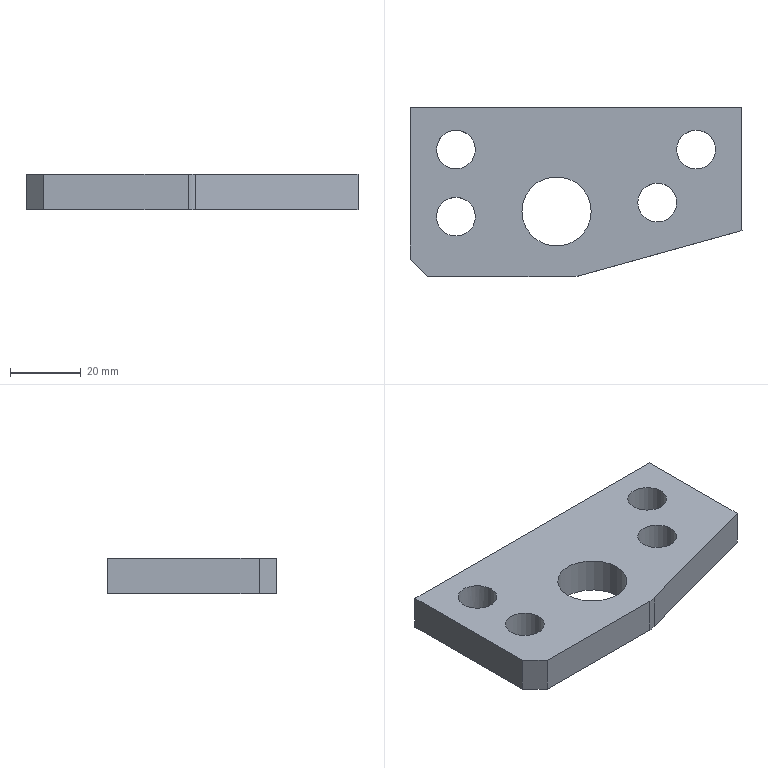Part | STEP file | lll_id4514_x_t | 1 solid | 14 faces | box 94 x 48 x 10 mm | volume 35108 mm3 | plane 8 | cylinder 6 | commonest cylinder face diameters 11 x4 16 x1 19.6 x1
STEP:
#1=CARTESIAN_POINT('',(3558.734,-207.45,-35.));
#2=VERTEX_POINT('',#1);
#3=CARTESIAN_POINT('',(3558.734,-212.95,-35.));
#4=DIRECTION('',(0.,0.,1.));
#5=DIRECTION('',(0.,1.,0.));
#6=AXIS2_PLACEMENT_3D('',#3,#4,#5);
#7=CIRCLE('',#6,5.5);
#8=EDGE_CURVE('',#2,#2,#7,.T.);
#9=ORIENTED_EDGE('',*,*,#8,.F.);
#10=EDGE_LOOP('',(#9));
#11=FACE_BOUND('',#10,.T.);
#12=CARTESIAN_POINT('',(3545.734,-200.95,-35.));
#13=VERTEX_POINT('',#12);
#14=CARTESIAN_POINT('',(3545.734,-243.95,-35.));
#15=VERTEX_POINT('',#14);
#16=CARTESIAN_POINT('',(3545.734,-198.7,-35.));
#17=DIRECTION('',(0.,-1.,0.));
#18=VECTOR('',#17,1.);
#19=LINE('',#16,#18);
#20=EDGE_CURVE('',#13,#15,#19,.T.);
#21=ORIENTED_EDGE('',*,*,#20,.T.);
#22=CARTESIAN_POINT('',(3550.734,-248.95,-35.));
#23=VERTEX_POINT('',#22);
#24=CARTESIAN_POINT('',(3540.359,-238.575,-35.));
#25=DIRECTION('',(0.7071,-0.7071,0.));
#26=VECTOR('',#25,1.);
#27=LINE('',#24,#26);
#28=EDGE_CURVE('',#15,#23,#27,.T.);
#29=ORIENTED_EDGE('',*,*,#28,.T.);
#30=CARTESIAN_POINT('',(3591.644,-248.95,-35.));
#31=VERTEX_POINT('',#30);
#32=CARTESIAN_POINT('',(3580.234,-248.95,-35.));
#33=DIRECTION('',(1.,0.,0.));
#34=VECTOR('',#33,1.);
#35=LINE('',#32,#34);
#36=EDGE_CURVE('',#23,#31,#35,.T.);
#37=ORIENTED_EDGE('',*,*,#36,.T.);
#38=CARTESIAN_POINT('',(3593.785,-248.658,-35.));
#39=VERTEX_POINT('',#38);
#40=CARTESIAN_POINT('',(3591.644,-240.95,-35.));
#41=DIRECTION('',(0.,0.,1.));
#42=DIRECTION('',(1.,0.,0.));
#43=AXIS2_PLACEMENT_3D('',#40,#41,#42);
#44=CIRCLE('',#43,8.);
#45=EDGE_CURVE('',#31,#39,#44,.T.);
#46=ORIENTED_EDGE('',*,*,#45,.T.);
#47=CARTESIAN_POINT('',(3639.734,-235.894,-35.));
#48=VERTEX_POINT('',#47);
#49=CARTESIAN_POINT('',(3594.088,-248.574,-35.));
#50=DIRECTION('',(0.9635,0.2676,0.));
#51=VECTOR('',#50,1.);
#52=LINE('',#49,#51);
#53=EDGE_CURVE('',#39,#48,#52,.T.);
#54=ORIENTED_EDGE('',*,*,#53,.T.);
#55=CARTESIAN_POINT('',(3639.734,-200.95,-35.));
#56=VERTEX_POINT('',#55);
#57=CARTESIAN_POINT('',(3639.734,-198.7,-35.));
#58=DIRECTION('',(0.,1.,0.));
#59=VECTOR('',#58,1.);
#60=LINE('',#57,#59);
#61=EDGE_CURVE('',#48,#56,#60,.T.);
#62=ORIENTED_EDGE('',*,*,#61,.T.);
#63=CARTESIAN_POINT('',(3580.234,-200.95,-35.));
#64=DIRECTION('',(-1.,0.,0.));
#65=VECTOR('',#64,1.);
#66=LINE('',#63,#65);
#67=EDGE_CURVE('',#56,#13,#66,.T.);
#68=ORIENTED_EDGE('',*,*,#67,.T.);
#69=EDGE_LOOP('',(#21,#29,#37,#46,#54,#62,#68));
#70=FACE_BOUND('',#69,.T.);
#71=CARTESIAN_POINT('',(3553.234,-231.95,-35.));
#72=VERTEX_POINT('',#71);
#73=CARTESIAN_POINT('',(3558.734,-231.95,-35.));
#74=DIRECTION('',(0.,0.,1.));
#75=DIRECTION('',(-1.,0.,0.));
#76=AXIS2_PLACEMENT_3D('',#73,#74,#75);
#77=CIRCLE('',#76,5.5);
#78=EDGE_CURVE('',#72,#72,#77,.T.);
#79=ORIENTED_EDGE('',*,*,#78,.F.);
#80=EDGE_LOOP('',(#79));
#81=FACE_BOUND('',#80,.T.);
#82=CARTESIAN_POINT('',(3610.234,-227.95,-35.));
#83=VERTEX_POINT('',#82);
#84=CARTESIAN_POINT('',(3615.734,-227.95,-35.));
#85=DIRECTION('',(0.,0.,1.));
#86=DIRECTION('',(-1.,0.,0.));
#87=AXIS2_PLACEMENT_3D('',#84,#85,#86);
#88=CIRCLE('',#87,5.5);
#89=EDGE_CURVE('',#83,#83,#88,.T.);
#90=ORIENTED_EDGE('',*,*,#89,.F.);
#91=EDGE_LOOP('',(#90));
#92=FACE_BOUND('',#91,.T.);
#93=CARTESIAN_POINT('',(3632.234,-212.95,-35.));
#94=VERTEX_POINT('',#93);
#95=CARTESIAN_POINT('',(3626.734,-212.95,-35.));
#96=DIRECTION('',(0.,0.,1.));
#97=DIRECTION('',(1.,0.,0.));
#98=AXIS2_PLACEMENT_3D('',#95,#96,#97);
#99=CIRCLE('',#98,5.5);
#100=EDGE_CURVE('',#94,#94,#99,.T.);
#101=ORIENTED_EDGE('',*,*,#100,.F.);
#102=EDGE_LOOP('',(#101));
#103=FACE_BOUND('',#102,.T.);
#104=CARTESIAN_POINT('',(3597.034,-230.45,-35.));
#105=VERTEX_POINT('',#104);
#106=CARTESIAN_POINT('',(3587.234,-230.45,-35.));
#107=DIRECTION('',(0.,0.,-1.));
#108=DIRECTION('',(1.,0.,0.));
#109=AXIS2_PLACEMENT_3D('',#106,#107,#108);
#110=CIRCLE('',#109,9.8);
#111=EDGE_CURVE('',#105,#105,#110,.T.);
#112=ORIENTED_EDGE('',*,*,#111,.T.);
#113=EDGE_LOOP('',(#112));
#114=FACE_BOUND('',#113,.T.);
#115=CARTESIAN_POINT('',(3580.234,-198.7,-35.));
#116=DIRECTION('',(0.,0.,-1.));
#117=DIRECTION('',(0.,-1.,0.));
#118=AXIS2_PLACEMENT_3D('',#115,#116,#117);
#119=PLANE('',#118);
#120=ADVANCED_FACE('',(#11,#70,#81,#92,#103,#114),#119,.F.);
#121=CARTESIAN_POINT('',(3564.234,-212.95,-45.));
#122=VERTEX_POINT('',#121);
#123=CARTESIAN_POINT('',(3558.734,-212.95,-45.));
#124=DIRECTION('',(0.,0.,1.));
#125=DIRECTION('',(1.,0.,0.));
#126=AXIS2_PLACEMENT_3D('',#123,#124,#125);
#127=CIRCLE('',#126,5.5);
#128=EDGE_CURVE('',#122,#122,#127,.T.);
#129=ORIENTED_EDGE('',*,*,#128,.T.);
#130=EDGE_LOOP('',(#129));
#131=FACE_BOUND('',#130,.T.);
#132=CARTESIAN_POINT('',(3545.734,-200.95,-45.));
#133=VERTEX_POINT('',#132);
#134=CARTESIAN_POINT('',(3545.734,-243.95,-45.));
#135=VERTEX_POINT('',#134);
#136=CARTESIAN_POINT('',(3545.734,-198.7,-45.));
#137=DIRECTION('',(0.,-1.,0.));
#138=VECTOR('',#137,1.);
#139=LINE('',#136,#138);
#140=EDGE_CURVE('',#133,#135,#139,.T.);
#141=ORIENTED_EDGE('',*,*,#140,.F.);
#142=CARTESIAN_POINT('',(3639.734,-200.95,-45.));
#143=VERTEX_POINT('',#142);
#144=CARTESIAN_POINT('',(3580.234,-200.95,-45.));
#145=DIRECTION('',(-1.,0.,0.));
#146=VECTOR('',#145,1.);
#147=LINE('',#144,#146);
#148=EDGE_CURVE('',#143,#133,#147,.T.);
#149=ORIENTED_EDGE('',*,*,#148,.F.);
#150=CARTESIAN_POINT('',(3639.734,-235.894,-45.));
#151=VERTEX_POINT('',#150);
#152=CARTESIAN_POINT('',(3639.734,-198.7,-45.));
#153=DIRECTION('',(0.,1.,0.));
#154=VECTOR('',#153,1.);
#155=LINE('',#152,#154);
#156=EDGE_CURVE('',#151,#143,#155,.T.);
#157=ORIENTED_EDGE('',*,*,#156,.F.);
#158=CARTESIAN_POINT('',(3593.785,-248.658,-45.));
#159=VERTEX_POINT('',#158);
#160=CARTESIAN_POINT('',(3594.088,-248.574,-45.));
#161=DIRECTION('',(0.9635,0.2676,0.));
#162=VECTOR('',#161,1.);
#163=LINE('',#160,#162);
#164=EDGE_CURVE('',#159,#151,#163,.T.);
#165=ORIENTED_EDGE('',*,*,#164,.F.);
#166=CARTESIAN_POINT('',(3591.644,-248.95,-45.));
#167=VERTEX_POINT('',#166);
#168=CARTESIAN_POINT('',(3591.644,-240.95,-45.));
#169=DIRECTION('',(0.,0.,1.));
#170=DIRECTION('',(1.,0.,0.));
#171=AXIS2_PLACEMENT_3D('',#168,#169,#170);
#172=CIRCLE('',#171,8.);
#173=EDGE_CURVE('',#167,#159,#172,.T.);
#174=ORIENTED_EDGE('',*,*,#173,.F.);
#175=CARTESIAN_POINT('',(3550.734,-248.95,-45.));
#176=VERTEX_POINT('',#175);
#177=CARTESIAN_POINT('',(3580.234,-248.95,-45.));
#178=DIRECTION('',(1.,0.,0.));
#179=VECTOR('',#178,1.);
#180=LINE('',#177,#179);
#181=EDGE_CURVE('',#176,#167,#180,.T.);
#182=ORIENTED_EDGE('',*,*,#181,.F.);
#183=CARTESIAN_POINT('',(3540.359,-238.575,-45.));
#184=DIRECTION('',(0.7071,-0.7071,0.));
#185=VECTOR('',#184,1.);
#186=LINE('',#183,#185);
#187=EDGE_CURVE('',#135,#176,#186,.T.);
#188=ORIENTED_EDGE('',*,*,#187,.F.);
#189=EDGE_LOOP('',(#141,#149,#157,#165,#174,#182,#188));
#190=FACE_BOUND('',#189,.T.);
#191=CARTESIAN_POINT('',(3553.234,-231.95,-45.));
#192=VERTEX_POINT('',#191);
#193=CARTESIAN_POINT('',(3558.734,-231.95,-45.));
#194=DIRECTION('',(0.,0.,1.));
#195=DIRECTION('',(-1.,0.,0.));
#196=AXIS2_PLACEMENT_3D('',#193,#194,#195);
#197=CIRCLE('',#196,5.5);
#198=EDGE_CURVE('',#192,#192,#197,.T.);
#199=ORIENTED_EDGE('',*,*,#198,.T.);
#200=EDGE_LOOP('',(#199));
#201=FACE_BOUND('',#200,.T.);
#202=CARTESIAN_POINT('',(3610.234,-227.95,-45.));
#203=VERTEX_POINT('',#202);
#204=CARTESIAN_POINT('',(3615.734,-227.95,-45.));
#205=DIRECTION('',(0.,0.,1.));
#206=DIRECTION('',(-1.,0.,0.));
#207=AXIS2_PLACEMENT_3D('',#204,#205,#206);
#208=CIRCLE('',#207,5.5);
#209=EDGE_CURVE('',#203,#203,#208,.T.);
#210=ORIENTED_EDGE('',*,*,#209,.T.);
#211=EDGE_LOOP('',(#210));
#212=FACE_BOUND('',#211,.T.);
#213=CARTESIAN_POINT('',(3632.234,-212.95,-45.));
#214=VERTEX_POINT('',#213);
#215=CARTESIAN_POINT('',(3626.734,-212.95,-45.));
#216=DIRECTION('',(0.,0.,1.));
#217=DIRECTION('',(1.,0.,0.));
#218=AXIS2_PLACEMENT_3D('',#215,#216,#217);
#219=CIRCLE('',#218,5.5);
#220=EDGE_CURVE('',#214,#214,#219,.T.);
#221=ORIENTED_EDGE('',*,*,#220,.T.);
#222=EDGE_LOOP('',(#221));
#223=FACE_BOUND('',#222,.T.);
#224=CARTESIAN_POINT('',(3597.034,-230.45,-45.));
#225=VERTEX_POINT('',#224);
#226=CARTESIAN_POINT('',(3587.234,-230.45,-45.));
#227=DIRECTION('',(0.,0.,-1.));
#228=DIRECTION('',(1.,0.,0.));
#229=AXIS2_PLACEMENT_3D('',#226,#227,#228);
#230=CIRCLE('',#229,9.8);
#231=EDGE_CURVE('',#225,#225,#230,.T.);
#232=ORIENTED_EDGE('',*,*,#231,.F.);
#233=EDGE_LOOP('',(#232));
#234=FACE_BOUND('',#233,.T.);
#235=CARTESIAN_POINT('',(3580.234,-198.7,-45.));
#236=DIRECTION('',(0.,0.,-1.));
#237=DIRECTION('',(0.,-1.,0.));
#238=AXIS2_PLACEMENT_3D('',#235,#236,#237);
#239=PLANE('',#238);
#240=ADVANCED_FACE('',(#131,#190,#201,#212,#223,#234),#239,.T.);
#241=CARTESIAN_POINT('',(3550.734,-248.95,-35.));
#242=DIRECTION('',(0.,0.,1.));
#243=VECTOR('',#242,1.);
#244=LINE('',#241,#243);
#245=EDGE_CURVE('',#176,#23,#244,.T.);
#246=ORIENTED_EDGE('',*,*,#245,.F.);
#247=ORIENTED_EDGE('',*,*,#181,.T.);
#248=CARTESIAN_POINT('',(3591.644,-248.95,-35.));
#249=DIRECTION('',(0.,0.,1.));
#250=VECTOR('',#249,1.);
#251=LINE('',#248,#250);
#252=EDGE_CURVE('',#167,#31,#251,.T.);
#253=ORIENTED_EDGE('',*,*,#252,.T.);
#254=ORIENTED_EDGE('',*,*,#36,.F.);
#255=EDGE_LOOP('',(#246,#247,#253,#254));
#256=FACE_OUTER_BOUND('',#255,.T.);
#257=CARTESIAN_POINT('',(3580.234,-248.95,-35.));
#258=DIRECTION('',(0.,-1.,0.));
#259=DIRECTION('',(1.,0.,0.));
#260=AXIS2_PLACEMENT_3D('',#257,#258,#259);
#261=PLANE('',#260);
#262=ADVANCED_FACE('',(#256),#261,.T.);
#263=ORIENTED_EDGE('',*,*,#252,.F.);
#264=ORIENTED_EDGE('',*,*,#173,.T.);
#265=CARTESIAN_POINT('',(3593.785,-248.658,-35.));
#266=DIRECTION('',(0.,0.,1.));
#267=VECTOR('',#266,1.);
#268=LINE('',#265,#267);
#269=EDGE_CURVE('',#159,#39,#268,.T.);
#270=ORIENTED_EDGE('',*,*,#269,.T.);
#271=ORIENTED_EDGE('',*,*,#45,.F.);
#272=EDGE_LOOP('',(#263,#264,#270,#271));
#273=FACE_OUTER_BOUND('',#272,.T.);
#274=CARTESIAN_POINT('',(3591.644,-240.95,-35.));
#275=DIRECTION('',(0.,0.,-1.));
#276=DIRECTION('',(1.,0.,0.));
#277=AXIS2_PLACEMENT_3D('',#274,#275,#276);
#278=CYLINDRICAL_SURFACE('',#277,8.);
#279=ADVANCED_FACE('',(#273),#278,.T.);
#280=ORIENTED_EDGE('',*,*,#269,.F.);
#281=ORIENTED_EDGE('',*,*,#164,.T.);
#282=CARTESIAN_POINT('',(3639.734,-235.894,-35.));
#283=DIRECTION('',(0.,0.,1.));
#284=VECTOR('',#283,1.);
#285=LINE('',#282,#284);
#286=EDGE_CURVE('',#151,#48,#285,.T.);
#287=ORIENTED_EDGE('',*,*,#286,.T.);
#288=ORIENTED_EDGE('',*,*,#53,.F.);
#289=EDGE_LOOP('',(#280,#281,#287,#288));
#290=FACE_OUTER_BOUND('',#289,.T.);
#291=CARTESIAN_POINT('',(3594.088,-248.574,-35.));
#292=DIRECTION('',(-0.2676,0.9635,0.));
#293=DIRECTION('',(-0.9635,-0.2676,0.));
#294=AXIS2_PLACEMENT_3D('',#291,#292,#293);
#295=PLANE('',#294);
#296=ADVANCED_FACE('',(#290),#295,.F.);
#297=ORIENTED_EDGE('',*,*,#286,.F.);
#298=ORIENTED_EDGE('',*,*,#156,.T.);
#299=CARTESIAN_POINT('',(3639.734,-200.95,-35.));
#300=DIRECTION('',(0.,0.,1.));
#301=VECTOR('',#300,1.);
#302=LINE('',#299,#301);
#303=EDGE_CURVE('',#143,#56,#302,.T.);
#304=ORIENTED_EDGE('',*,*,#303,.T.);
#305=ORIENTED_EDGE('',*,*,#61,.F.);
#306=EDGE_LOOP('',(#297,#298,#304,#305));
#307=FACE_OUTER_BOUND('',#306,.T.);
#308=CARTESIAN_POINT('',(3639.734,-198.7,-35.));
#309=DIRECTION('',(1.,0.,0.));
#310=DIRECTION('',(0.,1.,0.));
#311=AXIS2_PLACEMENT_3D('',#308,#309,#310);
#312=PLANE('',#311);
#313=ADVANCED_FACE('',(#307),#312,.T.);
#314=ORIENTED_EDGE('',*,*,#303,.F.);
#315=ORIENTED_EDGE('',*,*,#148,.T.);
#316=CARTESIAN_POINT('',(3545.734,-200.95,-35.));
#317=DIRECTION('',(0.,0.,1.));
#318=VECTOR('',#317,1.);
#319=LINE('',#316,#318);
#320=EDGE_CURVE('',#133,#13,#319,.T.);
#321=ORIENTED_EDGE('',*,*,#320,.T.);
#322=ORIENTED_EDGE('',*,*,#67,.F.);
#323=EDGE_LOOP('',(#314,#315,#321,#322));
#324=FACE_OUTER_BOUND('',#323,.T.);
#325=CARTESIAN_POINT('',(3580.234,-200.95,-35.));
#326=DIRECTION('',(0.,1.,0.));
#327=DIRECTION('',(-1.,0.,0.));
#328=AXIS2_PLACEMENT_3D('',#325,#326,#327);
#329=PLANE('',#328);
#330=ADVANCED_FACE('',(#324),#329,.T.);
#331=ORIENTED_EDGE('',*,*,#320,.F.);
#332=ORIENTED_EDGE('',*,*,#140,.T.);
#333=CARTESIAN_POINT('',(3545.734,-243.95,-35.));
#334=DIRECTION('',(0.,0.,1.));
#335=VECTOR('',#334,1.);
#336=LINE('',#333,#335);
#337=EDGE_CURVE('',#135,#15,#336,.T.);
#338=ORIENTED_EDGE('',*,*,#337,.T.);
#339=ORIENTED_EDGE('',*,*,#20,.F.);
#340=EDGE_LOOP('',(#331,#332,#338,#339));
#341=FACE_OUTER_BOUND('',#340,.T.);
#342=CARTESIAN_POINT('',(3545.734,-198.7,-35.));
#343=DIRECTION('',(-1.,0.,0.));
#344=DIRECTION('',(0.,-1.,0.));
#345=AXIS2_PLACEMENT_3D('',#342,#343,#344);
#346=PLANE('',#345);
#347=ADVANCED_FACE('',(#341),#346,.T.);
#348=ORIENTED_EDGE('',*,*,#100,.T.);
#349=EDGE_LOOP('',(#348));
#350=FACE_BOUND('',#349,.T.);
#351=ORIENTED_EDGE('',*,*,#220,.F.);
#352=EDGE_LOOP('',(#351));
#353=FACE_BOUND('',#352,.T.);
#354=CARTESIAN_POINT('',(3626.734,-212.95,-35.));
#355=DIRECTION('',(0.,0.,-1.));
#356=DIRECTION('',(1.,0.,0.));
#357=AXIS2_PLACEMENT_3D('',#354,#355,#356);
#358=CYLINDRICAL_SURFACE('',#357,5.5);
#359=ADVANCED_FACE('',(#350,#353),#358,.F.);
#360=ORIENTED_EDGE('',*,*,#89,.T.);
#361=EDGE_LOOP('',(#360));
#362=FACE_BOUND('',#361,.T.);
#363=ORIENTED_EDGE('',*,*,#209,.F.);
#364=EDGE_LOOP('',(#363));
#365=FACE_BOUND('',#364,.T.);
#366=CARTESIAN_POINT('',(3615.734,-227.95,-35.));
#367=DIRECTION('',(0.,0.,-1.));
#368=DIRECTION('',(1.,0.,0.));
#369=AXIS2_PLACEMENT_3D('',#366,#367,#368);
#370=CYLINDRICAL_SURFACE('',#369,5.5);
#371=ADVANCED_FACE('',(#362,#365),#370,.F.);
#372=ORIENTED_EDGE('',*,*,#78,.T.);
#373=EDGE_LOOP('',(#372));
#374=FACE_BOUND('',#373,.T.);
#375=ORIENTED_EDGE('',*,*,#198,.F.);
#376=EDGE_LOOP('',(#375));
#377=FACE_BOUND('',#376,.T.);
#378=CARTESIAN_POINT('',(3558.734,-231.95,-35.));
#379=DIRECTION('',(0.,0.,1.));
#380=DIRECTION('',(-1.,0.,0.));
#381=AXIS2_PLACEMENT_3D('',#378,#379,#380);
#382=CYLINDRICAL_SURFACE('',#381,5.5);
#383=ADVANCED_FACE('',(#374,#377),#382,.F.);
#384=ORIENTED_EDGE('',*,*,#187,.T.);
#385=ORIENTED_EDGE('',*,*,#245,.T.);
#386=ORIENTED_EDGE('',*,*,#28,.F.);
#387=ORIENTED_EDGE('',*,*,#337,.F.);
#388=EDGE_LOOP('',(#384,#385,#386,#387));
#389=FACE_OUTER_BOUND('',#388,.T.);
#390=CARTESIAN_POINT('',(3540.359,-238.575,-35.));
#391=DIRECTION('',(0.7071,0.7071,0.));
#392=DIRECTION('',(-0.7071,0.7071,0.));
#393=AXIS2_PLACEMENT_3D('',#390,#391,#392);
#394=PLANE('',#393);
#395=ADVANCED_FACE('',(#389),#394,.F.);
#396=ORIENTED_EDGE('',*,*,#8,.T.);
#397=EDGE_LOOP('',(#396));
#398=FACE_BOUND('',#397,.T.);
#399=ORIENTED_EDGE('',*,*,#128,.F.);
#400=EDGE_LOOP('',(#399));
#401=FACE_BOUND('',#400,.T.);
#402=CARTESIAN_POINT('',(3558.734,-212.95,-35.));
#403=DIRECTION('',(0.,0.,-1.));
#404=DIRECTION('',(1.,0.,0.));
#405=AXIS2_PLACEMENT_3D('',#402,#403,#404);
#406=CYLINDRICAL_SURFACE('',#405,5.5);
#407=ADVANCED_FACE('',(#398,#401),#406,.F.);
#408=ORIENTED_EDGE('',*,*,#231,.T.);
#409=EDGE_LOOP('',(#408));
#410=FACE_BOUND('',#409,.T.);
#411=ORIENTED_EDGE('',*,*,#111,.F.);
#412=EDGE_LOOP('',(#411));
#413=FACE_BOUND('',#412,.T.);
#414=CARTESIAN_POINT('',(3587.234,-230.45,15.));
#415=DIRECTION('',(0.,0.,-1.));
#416=DIRECTION('',(1.,0.,0.));
#417=AXIS2_PLACEMENT_3D('',#414,#415,#416);
#418=CYLINDRICAL_SURFACE('',#417,9.8);
#419=ADVANCED_FACE('',(#410,#413),#418,.F.);
#420=CLOSED_SHELL('',(#120,#240,#262,#279,#296,#313,#330,#347,#359,#371,#383,#395,#407,#419));
#421=MANIFOLD_SOLID_BREP('',#420);
#422=(LENGTH_UNIT()NAMED_UNIT(*)SI_UNIT(.MILLI.,.METRE.));
#423=UNCERTAINTY_MEASURE_WITH_UNIT(LENGTH_MEASURE(0.00002),#422,'','');
#424=(NAMED_UNIT(*)PLANE_ANGLE_UNIT()SI_UNIT($,.RADIAN.));
#425=PLANE_ANGLE_MEASURE_WITH_UNIT(PLANE_ANGLE_MEASURE(0.01745),#424);
#426=DIMENSIONAL_EXPONENTS(0.,0.,0.,0.,0.,0.,0.);
#427=(CONVERSION_BASED_UNIT('DEGREE',#425)NAMED_UNIT(#426)PLANE_ANGLE_UNIT());
#428=(NAMED_UNIT(*)SI_UNIT($,.STERADIAN.)SOLID_ANGLE_UNIT());
#429=(GEOMETRIC_REPRESENTATION_CONTEXT(3)GLOBAL_UNCERTAINTY_ASSIGNED_CONTEXT((#423))GLOBAL_UNIT_ASSIGNED_CONTEXT((#422,#427,#428))REPRESENTATION_CONTEXT('',''));
#430=ADVANCED_BREP_SHAPE_REPRESENTATION('',(#421),#429);